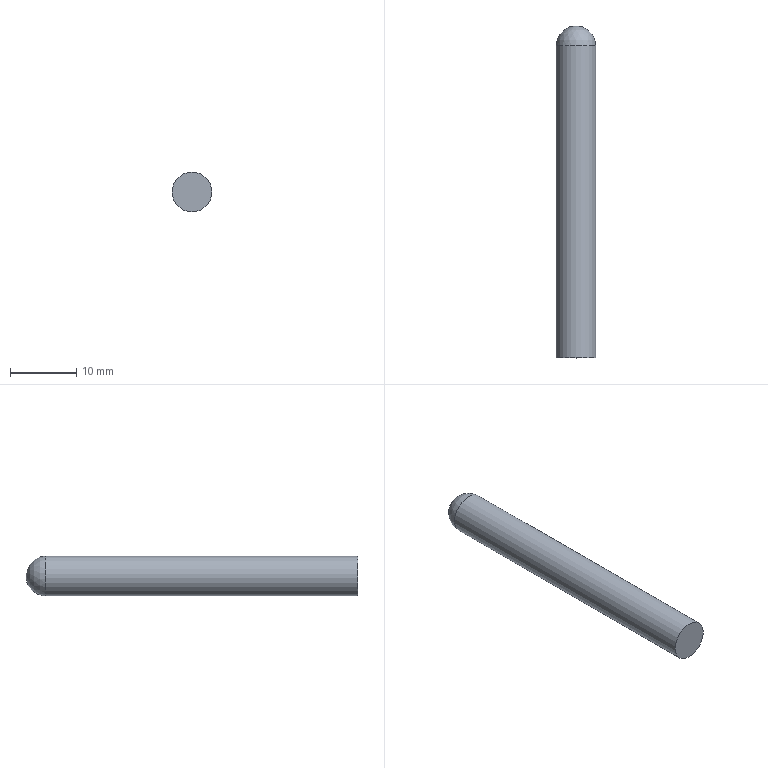Part | NX | features MFD10-WL40_4 2 | 1 solid | 3 faces | box 6 x 50 x 6 mm | volume 1385 mm3 | sphere 1 | cylinder 1 | plane 1 | commonest cylinder face diameters 6 x1
STEP:
#1=CARTESIAN_POINT('',(275.029,-418.95,84.95));
#2=VERTEX_POINT('',#1);
#3=CARTESIAN_POINT('',(275.029,-418.95,87.95));
#4=DIRECTION('',(0.,1.,0.));
#5=DIRECTION('',(0.,0.,-1.));
#6=AXIS2_PLACEMENT_3D('',#3,#4,#5);
#7=CIRCLE('',#6,3.);
#8=EDGE_CURVE('',#2,#2,#7,.T.);
#9=ORIENTED_EDGE('',*,*,#8,.T.);
#10=EDGE_LOOP('',(#9));
#11=FACE_BOUND('',#10,.T.);
#12=CARTESIAN_POINT('',(275.029,-418.95,87.95));
#13=DIRECTION('',(0.,-1.,0.));
#14=DIRECTION('',(0.,0.,-1.));
#15=AXIS2_PLACEMENT_3D('',#12,#13,#14);
#16=SPHERICAL_SURFACE('',#15,3.);
#17=ADVANCED_FACE('',(#11),#16,.T.);
#18=ORIENTED_EDGE('',*,*,#8,.F.);
#19=EDGE_LOOP('',(#18));
#20=FACE_BOUND('',#19,.T.);
#21=CARTESIAN_POINT('',(275.029,-465.95,84.95));
#22=VERTEX_POINT('',#21);
#23=CARTESIAN_POINT('',(275.029,-465.95,87.95));
#24=DIRECTION('',(0.,-1.,0.));
#25=DIRECTION('',(0.,0.,-1.));
#26=AXIS2_PLACEMENT_3D('',#23,#24,#25);
#27=CIRCLE('',#26,3.);
#28=EDGE_CURVE('',#22,#22,#27,.T.);
#29=ORIENTED_EDGE('',*,*,#28,.F.);
#30=EDGE_LOOP('',(#29));
#31=FACE_BOUND('',#30,.T.);
#32=CARTESIAN_POINT('',(275.029,-382.45,87.95));
#33=DIRECTION('',(0.,-1.,0.));
#34=DIRECTION('',(0.,0.,-1.));
#35=AXIS2_PLACEMENT_3D('',#32,#33,#34);
#36=CYLINDRICAL_SURFACE('',#35,3.);
#37=ADVANCED_FACE('',(#20,#31),#36,.T.);
#38=ORIENTED_EDGE('',*,*,#28,.T.);
#39=EDGE_LOOP('',(#38));
#40=FACE_BOUND('',#39,.T.);
#41=CARTESIAN_POINT('',(275.029,-465.95,87.95));
#42=DIRECTION('',(0.,-1.,0.));
#43=DIRECTION('',(0.,0.,-1.));
#44=AXIS2_PLACEMENT_3D('',#41,#42,#43);
#45=PLANE('',#44);
#46=ADVANCED_FACE('',(#40),#45,.T.);
#47=CLOSED_SHELL('',(#17,#37,#46));
#48=MANIFOLD_SOLID_BREP('',#47);
#49=(LENGTH_UNIT()NAMED_UNIT(*)SI_UNIT(.MILLI.,.METRE.));
#50=UNCERTAINTY_MEASURE_WITH_UNIT(LENGTH_MEASURE(0.00001),#49,'','');
#51=(NAMED_UNIT(*)PLANE_ANGLE_UNIT()SI_UNIT($,.RADIAN.));
#52=(NAMED_UNIT(*)SI_UNIT($,.STERADIAN.)SOLID_ANGLE_UNIT());
#53=(GEOMETRIC_REPRESENTATION_CONTEXT(3)GLOBAL_UNCERTAINTY_ASSIGNED_CONTEXT((#50))GLOBAL_UNIT_ASSIGNED_CONTEXT((#49,#51,#52))REPRESENTATION_CONTEXT('',''));
#54=ADVANCED_BREP_SHAPE_REPRESENTATION('',(#48),#53);